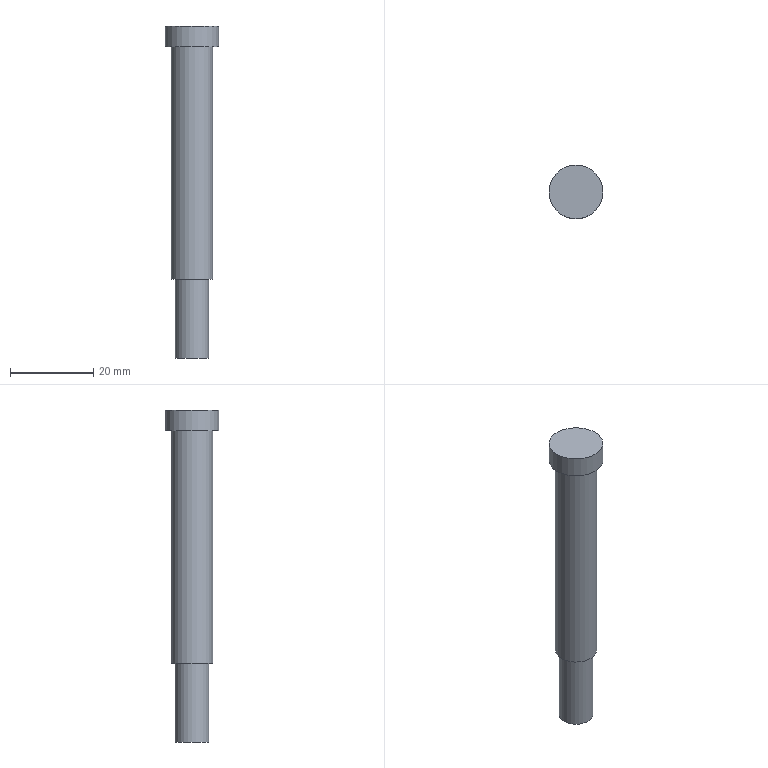Part | NX | features solid 2 | 1 solid | 7 faces | box 13 x 13 x 80 mm | volume 6041 mm3 | plane 4 | cylinder 3 | commonest cylinder face diameters 8.1 x1 10 x1 13 x1
STEP:
#1=CARTESIAN_POINT('',(-685.999,-287.091,43.));
#2=VERTEX_POINT('',#1);
#3=CARTESIAN_POINT('',(-690.999,-287.091,43.));
#4=DIRECTION('',(0.,0.,1.));
#5=DIRECTION('',(1.,0.,0.));
#6=AXIS2_PLACEMENT_3D('',#3,#4,#5);
#7=CIRCLE('',#6,5.);
#8=EDGE_CURVE('',#2,#2,#7,.T.);
#9=ORIENTED_EDGE('',*,*,#8,.T.);
#10=EDGE_LOOP('',(#9));
#11=FACE_BOUND('',#10,.T.);
#12=CARTESIAN_POINT('',(-685.999,-287.091,99.));
#13=VERTEX_POINT('',#12);
#14=CARTESIAN_POINT('',(-690.999,-287.091,99.));
#15=DIRECTION('',(0.,0.,1.));
#16=DIRECTION('',(1.,0.,0.));
#17=AXIS2_PLACEMENT_3D('',#14,#15,#16);
#18=CIRCLE('',#17,5.);
#19=EDGE_CURVE('',#13,#13,#18,.T.);
#20=ORIENTED_EDGE('',*,*,#19,.F.);
#21=EDGE_LOOP('',(#20));
#22=FACE_BOUND('',#21,.T.);
#23=CARTESIAN_POINT('',(-690.999,-287.091,104.));
#24=DIRECTION('',(0.,0.,-1.));
#25=DIRECTION('',(-1.,0.,0.));
#26=AXIS2_PLACEMENT_3D('',#23,#24,#25);
#27=CYLINDRICAL_SURFACE('',#26,5.);
#28=ADVANCED_FACE('',(#11,#22),#27,.T.);
#29=CARTESIAN_POINT('',(-686.949,-287.091,43.));
#30=VERTEX_POINT('',#29);
#31=CARTESIAN_POINT('',(-690.999,-287.091,43.));
#32=DIRECTION('',(0.,0.,1.));
#33=DIRECTION('',(1.,0.,0.));
#34=AXIS2_PLACEMENT_3D('',#31,#32,#33);
#35=CIRCLE('',#34,4.05);
#36=EDGE_CURVE('',#30,#30,#35,.T.);
#37=ORIENTED_EDGE('',*,*,#36,.T.);
#38=EDGE_LOOP('',(#37));
#39=FACE_BOUND('',#38,.T.);
#40=ORIENTED_EDGE('',*,*,#8,.F.);
#41=EDGE_LOOP('',(#40));
#42=FACE_BOUND('',#41,.T.);
#43=CARTESIAN_POINT('',(-690.999,-287.091,43.));
#44=DIRECTION('',(0.,0.,1.));
#45=DIRECTION('',(1.,0.,0.));
#46=AXIS2_PLACEMENT_3D('',#43,#44,#45);
#47=PLANE('',#46);
#48=ADVANCED_FACE('',(#39,#42),#47,.F.);
#49=CARTESIAN_POINT('',(-684.499,-287.091,99.));
#50=VERTEX_POINT('',#49);
#51=CARTESIAN_POINT('',(-690.999,-287.091,99.));
#52=DIRECTION('',(0.,0.,1.));
#53=DIRECTION('',(1.,0.,0.));
#54=AXIS2_PLACEMENT_3D('',#51,#52,#53);
#55=CIRCLE('',#54,6.5);
#56=EDGE_CURVE('',#50,#50,#55,.T.);
#57=ORIENTED_EDGE('',*,*,#56,.F.);
#58=EDGE_LOOP('',(#57));
#59=FACE_BOUND('',#58,.T.);
#60=ORIENTED_EDGE('',*,*,#19,.T.);
#61=EDGE_LOOP('',(#60));
#62=FACE_BOUND('',#61,.T.);
#63=CARTESIAN_POINT('',(-690.999,-287.091,99.));
#64=DIRECTION('',(0.,0.,1.));
#65=DIRECTION('',(1.,0.,0.));
#66=AXIS2_PLACEMENT_3D('',#63,#64,#65);
#67=PLANE('',#66);
#68=ADVANCED_FACE('',(#59,#62),#67,.F.);
#69=ORIENTED_EDGE('',*,*,#56,.T.);
#70=EDGE_LOOP('',(#69));
#71=FACE_BOUND('',#70,.T.);
#72=CARTESIAN_POINT('',(-684.499,-287.091,104.));
#73=VERTEX_POINT('',#72);
#74=CARTESIAN_POINT('',(-690.999,-287.091,104.));
#75=DIRECTION('',(0.,0.,1.));
#76=DIRECTION('',(1.,0.,0.));
#77=AXIS2_PLACEMENT_3D('',#74,#75,#76);
#78=CIRCLE('',#77,6.5);
#79=EDGE_CURVE('',#73,#73,#78,.T.);
#80=ORIENTED_EDGE('',*,*,#79,.F.);
#81=EDGE_LOOP('',(#80));
#82=FACE_BOUND('',#81,.T.);
#83=CARTESIAN_POINT('',(-690.999,-287.091,99.));
#84=DIRECTION('',(0.,0.,1.));
#85=DIRECTION('',(1.,0.,0.));
#86=AXIS2_PLACEMENT_3D('',#83,#84,#85);
#87=CYLINDRICAL_SURFACE('',#86,6.5);
#88=ADVANCED_FACE('',(#71,#82),#87,.T.);
#89=ORIENTED_EDGE('',*,*,#79,.T.);
#90=EDGE_LOOP('',(#89));
#91=FACE_BOUND('',#90,.T.);
#92=CARTESIAN_POINT('',(-690.999,-287.091,104.));
#93=DIRECTION('',(0.,0.,1.));
#94=DIRECTION('',(1.,0.,0.));
#95=AXIS2_PLACEMENT_3D('',#92,#93,#94);
#96=PLANE('',#95);
#97=ADVANCED_FACE('',(#91),#96,.T.);
#98=CARTESIAN_POINT('',(-686.949,-287.091,24.));
#99=VERTEX_POINT('',#98);
#100=CARTESIAN_POINT('',(-690.999,-287.091,24.));
#101=DIRECTION('',(0.,0.,1.));
#102=DIRECTION('',(1.,0.,0.));
#103=AXIS2_PLACEMENT_3D('',#100,#101,#102);
#104=CIRCLE('',#103,4.05);
#105=EDGE_CURVE('',#99,#99,#104,.T.);
#106=ORIENTED_EDGE('',*,*,#105,.T.);
#107=EDGE_LOOP('',(#106));
#108=FACE_BOUND('',#107,.T.);
#109=ORIENTED_EDGE('',*,*,#36,.F.);
#110=EDGE_LOOP('',(#109));
#111=FACE_BOUND('',#110,.T.);
#112=CARTESIAN_POINT('',(-690.999,-287.091,24.));
#113=DIRECTION('',(0.,0.,1.));
#114=DIRECTION('',(1.,0.,0.));
#115=AXIS2_PLACEMENT_3D('',#112,#113,#114);
#116=CYLINDRICAL_SURFACE('',#115,4.05);
#117=ADVANCED_FACE('',(#108,#111),#116,.T.);
#118=ORIENTED_EDGE('',*,*,#105,.F.);
#119=EDGE_LOOP('',(#118));
#120=FACE_BOUND('',#119,.T.);
#121=CARTESIAN_POINT('',(-690.999,-287.091,24.));
#122=DIRECTION('',(0.,0.,1.));
#123=DIRECTION('',(1.,0.,0.));
#124=AXIS2_PLACEMENT_3D('',#121,#122,#123);
#125=PLANE('',#124);
#126=ADVANCED_FACE('',(#120),#125,.F.);
#127=CLOSED_SHELL('',(#28,#48,#68,#88,#97,#117,#126));
#128=MANIFOLD_SOLID_BREP('',#127);
#129=(LENGTH_UNIT()NAMED_UNIT(*)SI_UNIT(.MILLI.,.METRE.));
#130=UNCERTAINTY_MEASURE_WITH_UNIT(LENGTH_MEASURE(0.00001),#129,'','');
#131=(NAMED_UNIT(*)PLANE_ANGLE_UNIT()SI_UNIT($,.RADIAN.));
#132=(NAMED_UNIT(*)SI_UNIT($,.STERADIAN.)SOLID_ANGLE_UNIT());
#133=(GEOMETRIC_REPRESENTATION_CONTEXT(3)GLOBAL_UNCERTAINTY_ASSIGNED_CONTEXT((#130))GLOBAL_UNIT_ASSIGNED_CONTEXT((#129,#131,#132))REPRESENTATION_CONTEXT('',''));
#134=ADVANCED_BREP_SHAPE_REPRESENTATION('',(#128),#133);